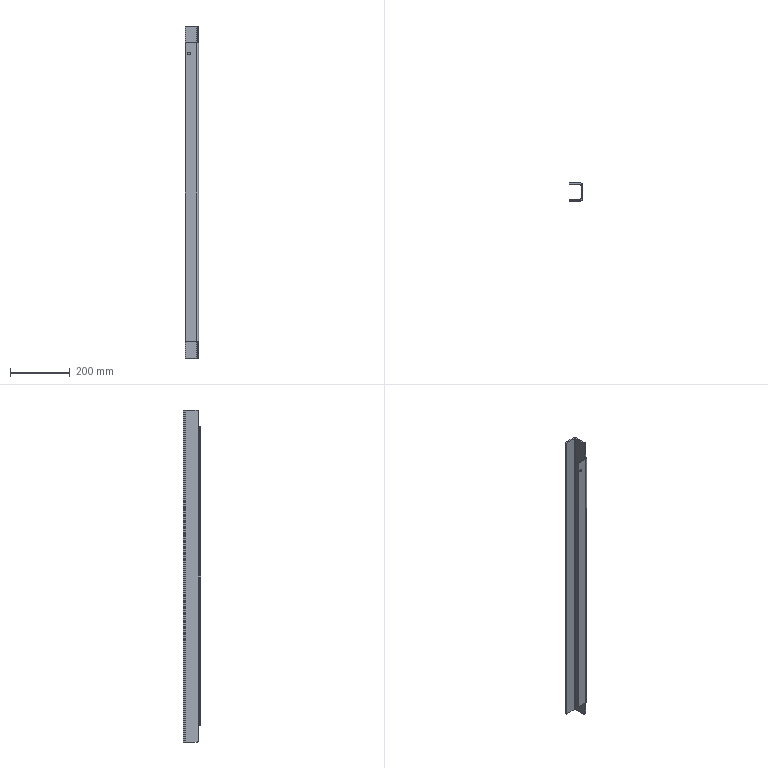Part | SolidWorks | features ICE 2, Extrusion 1, Fillet 1, HoleWzd 1 | 1 solid | 22 faces | box 45 x 60 x 1116 mm | volume 728504 mm3 | plane 14 | cylinder 8 | commonest cylinder face diameters 6 x2 8.5 x2 10 x2 16 x2
STEP:
#1=CARTESIAN_POINT('',(12.5,-60.,1028.25));
#2=VERTEX_POINT('',#1);
#3=CARTESIAN_POINT('',(12.5,-60.,1019.75));
#4=VERTEX_POINT('',#3);
#5=CARTESIAN_POINT('',(12.5,-60.,1024.));
#6=DIRECTION('',(0.,-1.,0.));
#7=DIRECTION('',(1.,0.,0.));
#8=AXIS2_PLACEMENT_3D('',#5,#6,#7);
#9=CIRCLE('',#8,4.25);
#10=EDGE_CURVE('',#2,#4,#9,.T.);
#11=ORIENTED_EDGE('',*,*,#10,.T.);
#12=CARTESIAN_POINT('',(12.5,-55.,1019.75));
#13=VERTEX_POINT('',#12);
#14=CARTESIAN_POINT('',(12.5,-55.,1019.75));
#15=DIRECTION('',(0.,1.,0.));
#16=VECTOR('',#15,1000.);
#17=LINE('',#14,#16);
#18=EDGE_CURVE('',#4,#13,#17,.T.);
#19=ORIENTED_EDGE('',*,*,#18,.T.);
#20=CARTESIAN_POINT('',(12.5,-55.,1028.25));
#21=VERTEX_POINT('',#20);
#22=CARTESIAN_POINT('',(12.5,-55.,1024.));
#23=DIRECTION('',(0.,1.,0.));
#24=DIRECTION('',(0.,0.,1.));
#25=AXIS2_PLACEMENT_3D('',#22,#23,#24);
#26=CIRCLE('',#25,4.25);
#27=EDGE_CURVE('',#13,#21,#26,.T.);
#28=ORIENTED_EDGE('',*,*,#27,.T.);
#29=CARTESIAN_POINT('',(12.5,-55.,1028.25));
#30=DIRECTION('',(0.,1.,0.));
#31=VECTOR('',#30,1000.);
#32=LINE('',#29,#31);
#33=EDGE_CURVE('',#2,#21,#32,.T.);
#34=ORIENTED_EDGE('',*,*,#33,.F.);
#35=EDGE_LOOP('',(#11,#19,#28,#34));
#36=FACE_OUTER_BOUND('',#35,.T.);
#37=CARTESIAN_POINT('',(12.5,-55.,1024.));
#38=DIRECTION('',(0.,1.,0.));
#39=DIRECTION('',(0.,0.,1.));
#40=AXIS2_PLACEMENT_3D('',#37,#38,#39);
#41=CYLINDRICAL_SURFACE('',#40,4.25);
#42=ADVANCED_FACE('',(#36),#41,.F.);
#43=CARTESIAN_POINT('',(12.5,-55.,1024.));
#44=DIRECTION('',(0.,1.,0.));
#45=DIRECTION('',(0.,0.,1.));
#46=AXIS2_PLACEMENT_3D('',#43,#44,#45);
#47=CIRCLE('',#46,4.25);
#48=EDGE_CURVE('',#21,#13,#47,.T.);
#49=ORIENTED_EDGE('',*,*,#48,.F.);
#50=ORIENTED_EDGE('',*,*,#27,.F.);
#51=EDGE_LOOP('',(#49,#50));
#52=FACE_BOUND('',#51,.T.);
#53=CARTESIAN_POINT('',(0.,-55.,1059.));
#54=VERTEX_POINT('',#53);
#55=CARTESIAN_POINT('',(0.,-55.,57.));
#56=VERTEX_POINT('',#55);
#57=CARTESIAN_POINT('',(0.,-55.,1116.));
#58=DIRECTION('',(0.,0.,-1.));
#59=VECTOR('',#58,1000.);
#60=LINE('',#57,#59);
#61=EDGE_CURVE('',#54,#56,#60,.T.);
#62=ORIENTED_EDGE('',*,*,#61,.F.);
#63=CARTESIAN_POINT('',(37.,-55.,1059.));
#64=VERTEX_POINT('',#63);
#65=CARTESIAN_POINT('',(37.,-55.,1059.));
#66=DIRECTION('',(1.,0.,0.));
#67=VECTOR('',#66,1000.);
#68=LINE('',#65,#67);
#69=EDGE_CURVE('',#54,#64,#68,.T.);
#70=ORIENTED_EDGE('',*,*,#69,.T.);
#71=CARTESIAN_POINT('',(37.,-55.,57.));
#72=VERTEX_POINT('',#71);
#73=CARTESIAN_POINT('',(37.,-55.,1116.));
#74=DIRECTION('',(0.,0.,-1.));
#75=VECTOR('',#74,1000.);
#76=LINE('',#73,#75);
#77=EDGE_CURVE('',#64,#72,#76,.T.);
#78=ORIENTED_EDGE('',*,*,#77,.T.);
#79=CARTESIAN_POINT('',(37.,-55.,57.));
#80=DIRECTION('',(-1.,0.,0.));
#81=VECTOR('',#80,1000.);
#82=LINE('',#79,#81);
#83=EDGE_CURVE('',#72,#56,#82,.T.);
#84=ORIENTED_EDGE('',*,*,#83,.T.);
#85=EDGE_LOOP('',(#62,#70,#78,#84));
#86=FACE_OUTER_BOUND('',#85,.T.);
#87=CARTESIAN_POINT('',(37.,-55.,1116.));
#88=DIRECTION('',(0.,-1.,0.));
#89=DIRECTION('',(0.,0.,-1.));
#90=AXIS2_PLACEMENT_3D('',#87,#88,#89);
#91=PLANE('',#90);
#92=ADVANCED_FACE('',(#52,#86),#91,.F.);
#93=CARTESIAN_POINT('',(0.,-60.,1059.));
#94=VERTEX_POINT('',#93);
#95=CARTESIAN_POINT('',(0.,-60.,57.));
#96=VERTEX_POINT('',#95);
#97=CARTESIAN_POINT('',(0.,-60.,1116.));
#98=DIRECTION('',(0.,0.,-1.));
#99=VECTOR('',#98,1000.);
#100=LINE('',#97,#99);
#101=EDGE_CURVE('',#94,#96,#100,.T.);
#102=ORIENTED_EDGE('',*,*,#101,.F.);
#103=CARTESIAN_POINT('',(0.,-52.,1059.));
#104=DIRECTION('',(0.,-1.,0.));
#105=VECTOR('',#104,1000.);
#106=LINE('',#103,#105);
#107=EDGE_CURVE('',#54,#94,#106,.T.);
#108=ORIENTED_EDGE('',*,*,#107,.F.);
#109=ORIENTED_EDGE('',*,*,#61,.T.);
#110=CARTESIAN_POINT('',(0.,-96.857,57.));
#111=DIRECTION('',(0.,1.,0.));
#112=VECTOR('',#111,1000.);
#113=LINE('',#110,#112);
#114=EDGE_CURVE('',#96,#56,#113,.T.);
#115=ORIENTED_EDGE('',*,*,#114,.F.);
#116=EDGE_LOOP('',(#102,#108,#109,#115));
#117=FACE_OUTER_BOUND('',#116,.T.);
#118=CARTESIAN_POINT('',(0.,-55.,1116.));
#119=DIRECTION('',(1.,0.,0.));
#120=DIRECTION('',(0.,0.,-1.));
#121=AXIS2_PLACEMENT_3D('',#118,#119,#120);
#122=PLANE('',#121);
#123=ADVANCED_FACE('',(#117),#122,.F.);
#124=ORIENTED_EDGE('',*,*,#10,.F.);
#125=CARTESIAN_POINT('',(12.5,-60.,1024.));
#126=DIRECTION('',(0.,-1.,0.));
#127=DIRECTION('',(1.,0.,0.));
#128=AXIS2_PLACEMENT_3D('',#125,#126,#127);
#129=CIRCLE('',#128,4.25);
#130=EDGE_CURVE('',#4,#2,#129,.T.);
#131=ORIENTED_EDGE('',*,*,#130,.F.);
#132=EDGE_LOOP('',(#124,#131));
#133=FACE_BOUND('',#132,.T.);
#134=CARTESIAN_POINT('',(37.,-60.,1059.));
#135=VERTEX_POINT('',#134);
#136=CARTESIAN_POINT('',(37.,-60.,1059.));
#137=DIRECTION('',(1.,0.,0.));
#138=VECTOR('',#137,1000.);
#139=LINE('',#136,#138);
#140=EDGE_CURVE('',#94,#135,#139,.T.);
#141=ORIENTED_EDGE('',*,*,#140,.F.);
#142=ORIENTED_EDGE('',*,*,#101,.T.);
#143=CARTESIAN_POINT('',(37.,-60.,57.));
#144=VERTEX_POINT('',#143);
#145=CARTESIAN_POINT('',(37.,-60.,57.));
#146=DIRECTION('',(-1.,0.,0.));
#147=VECTOR('',#146,1000.);
#148=LINE('',#145,#147);
#149=EDGE_CURVE('',#144,#96,#148,.T.);
#150=ORIENTED_EDGE('',*,*,#149,.F.);
#151=CARTESIAN_POINT('',(37.,-60.,1116.));
#152=DIRECTION('',(0.,0.,-1.));
#153=VECTOR('',#152,1000.);
#154=LINE('',#151,#153);
#155=EDGE_CURVE('',#135,#144,#154,.T.);
#156=ORIENTED_EDGE('',*,*,#155,.F.);
#157=EDGE_LOOP('',(#141,#142,#150,#156));
#158=FACE_OUTER_BOUND('',#157,.T.);
#159=CARTESIAN_POINT('',(37.,-60.,1116.));
#160=DIRECTION('',(0.,-1.,0.));
#161=DIRECTION('',(1.,0.,0.));
#162=AXIS2_PLACEMENT_3D('',#159,#160,#161);
#163=PLANE('',#162);
#164=ADVANCED_FACE('',(#133,#158),#163,.T.);
#165=CARTESIAN_POINT('',(45.,-52.,1059.));
#166=VERTEX_POINT('',#165);
#167=CARTESIAN_POINT('',(37.,-52.,1059.));
#168=DIRECTION('',(0.,0.,1.));
#169=DIRECTION('',(-1.,0.,0.));
#170=AXIS2_PLACEMENT_3D('',#167,#168,#169);
#171=CIRCLE('',#170,8.);
#172=EDGE_CURVE('',#135,#166,#171,.T.);
#173=ORIENTED_EDGE('',*,*,#172,.F.);
#174=ORIENTED_EDGE('',*,*,#155,.T.);
#175=CARTESIAN_POINT('',(45.,-52.,57.));
#176=VERTEX_POINT('',#175);
#177=CARTESIAN_POINT('',(37.,-52.,57.));
#178=DIRECTION('',(0.,0.,-1.));
#179=DIRECTION('',(1.,0.,0.));
#180=AXIS2_PLACEMENT_3D('',#177,#178,#179);
#181=CIRCLE('',#180,8.);
#182=EDGE_CURVE('',#176,#144,#181,.T.);
#183=ORIENTED_EDGE('',*,*,#182,.F.);
#184=CARTESIAN_POINT('',(45.,-52.,1116.));
#185=DIRECTION('',(0.,0.,-1.));
#186=VECTOR('',#185,1000.);
#187=LINE('',#184,#186);
#188=EDGE_CURVE('',#166,#176,#187,.T.);
#189=ORIENTED_EDGE('',*,*,#188,.F.);
#190=EDGE_LOOP('',(#173,#174,#183,#189));
#191=FACE_OUTER_BOUND('',#190,.T.);
#192=CARTESIAN_POINT('',(37.,-52.,1116.));
#193=DIRECTION('',(0.,0.,-1.));
#194=DIRECTION('',(-1.,0.,0.));
#195=AXIS2_PLACEMENT_3D('',#192,#193,#194);
#196=CYLINDRICAL_SURFACE('',#195,8.);
#197=ADVANCED_FACE('',(#191),#196,.T.);
#198=CARTESIAN_POINT('',(45.,-8.,1116.));
#199=VERTEX_POINT('',#198);
#200=CARTESIAN_POINT('',(45.,-47.,1116.));
#201=VERTEX_POINT('',#200);
#202=CARTESIAN_POINT('',(45.,-8.,1116.));
#203=DIRECTION('',(0.,-1.,0.));
#204=VECTOR('',#203,1000.);
#205=LINE('',#202,#204);
#206=EDGE_CURVE('',#199,#201,#205,.T.);
#207=ORIENTED_EDGE('',*,*,#206,.T.);
#208=CARTESIAN_POINT('',(45.,-52.,1111.));
#209=VERTEX_POINT('',#208);
#210=CARTESIAN_POINT('',(45.,-47.,1111.));
#211=DIRECTION('',(1.,0.,0.));
#212=DIRECTION('',(0.,1.,0.));
#213=AXIS2_PLACEMENT_3D('',#210,#211,#212);
#214=CIRCLE('',#213,5.);
#215=EDGE_CURVE('',#201,#209,#214,.T.);
#216=ORIENTED_EDGE('',*,*,#215,.T.);
#217=CARTESIAN_POINT('',(45.,-52.,1116.));
#218=DIRECTION('',(0.,0.,-1.));
#219=VECTOR('',#218,1000.);
#220=LINE('',#217,#219);
#221=EDGE_CURVE('',#209,#166,#220,.T.);
#222=ORIENTED_EDGE('',*,*,#221,.T.);
#223=ORIENTED_EDGE('',*,*,#188,.T.);
#224=CARTESIAN_POINT('',(45.,-52.,5.));
#225=VERTEX_POINT('',#224);
#226=CARTESIAN_POINT('',(45.,-52.,1116.));
#227=DIRECTION('',(0.,0.,1.));
#228=VECTOR('',#227,1000.);
#229=LINE('',#226,#228);
#230=EDGE_CURVE('',#225,#176,#229,.T.);
#231=ORIENTED_EDGE('',*,*,#230,.F.);
#232=CARTESIAN_POINT('',(45.,-47.,0.));
#233=VERTEX_POINT('',#232);
#234=CARTESIAN_POINT('',(45.,-47.,5.));
#235=DIRECTION('',(1.,0.,0.));
#236=DIRECTION('',(0.,1.,0.));
#237=AXIS2_PLACEMENT_3D('',#234,#235,#236);
#238=CIRCLE('',#237,5.);
#239=EDGE_CURVE('',#225,#233,#238,.T.);
#240=ORIENTED_EDGE('',*,*,#239,.T.);
#241=CARTESIAN_POINT('',(45.,-8.,0.));
#242=VERTEX_POINT('',#241);
#243=CARTESIAN_POINT('',(45.,-8.,0.));
#244=DIRECTION('',(0.,-1.,0.));
#245=VECTOR('',#244,1000.);
#246=LINE('',#243,#245);
#247=EDGE_CURVE('',#242,#233,#246,.T.);
#248=ORIENTED_EDGE('',*,*,#247,.F.);
#249=CARTESIAN_POINT('',(45.,-8.,1116.));
#250=DIRECTION('',(0.,0.,-1.));
#251=VECTOR('',#250,1000.);
#252=LINE('',#249,#251);
#253=EDGE_CURVE('',#199,#242,#252,.T.);
#254=ORIENTED_EDGE('',*,*,#253,.F.);
#255=EDGE_LOOP('',(#207,#216,#222,#223,#231,#240,#248,#254));
#256=FACE_OUTER_BOUND('',#255,.T.);
#257=CARTESIAN_POINT('',(45.,-8.,1116.));
#258=DIRECTION('',(1.,0.,0.));
#259=DIRECTION('',(0.,1.,0.));
#260=AXIS2_PLACEMENT_3D('',#257,#258,#259);
#261=PLANE('',#260);
#262=ADVANCED_FACE('',(#256),#261,.T.);
#263=CARTESIAN_POINT('',(37.,0.,0.));
#264=VERTEX_POINT('',#263);
#265=CARTESIAN_POINT('',(37.,-8.,0.));
#266=DIRECTION('',(0.,0.,-1.));
#267=DIRECTION('',(-1.,0.,0.));
#268=AXIS2_PLACEMENT_3D('',#265,#266,#267);
#269=CIRCLE('',#268,8.);
#270=EDGE_CURVE('',#264,#242,#269,.T.);
#271=ORIENTED_EDGE('',*,*,#270,.F.);
#272=CARTESIAN_POINT('',(37.,0.,1116.));
#273=VERTEX_POINT('',#272);
#274=CARTESIAN_POINT('',(37.,0.,1116.));
#275=DIRECTION('',(0.,0.,-1.));
#276=VECTOR('',#275,1000.);
#277=LINE('',#274,#276);
#278=EDGE_CURVE('',#273,#264,#277,.T.);
#279=ORIENTED_EDGE('',*,*,#278,.F.);
#280=CARTESIAN_POINT('',(37.,-8.,1116.));
#281=DIRECTION('',(0.,0.,-1.));
#282=DIRECTION('',(-1.,0.,0.));
#283=AXIS2_PLACEMENT_3D('',#280,#281,#282);
#284=CIRCLE('',#283,8.);
#285=EDGE_CURVE('',#273,#199,#284,.T.);
#286=ORIENTED_EDGE('',*,*,#285,.T.);
#287=ORIENTED_EDGE('',*,*,#253,.T.);
#288=EDGE_LOOP('',(#271,#279,#286,#287));
#289=FACE_OUTER_BOUND('',#288,.T.);
#290=CARTESIAN_POINT('',(37.,-8.,1116.));
#291=DIRECTION('',(0.,0.,-1.));
#292=DIRECTION('',(-1.,0.,0.));
#293=AXIS2_PLACEMENT_3D('',#290,#291,#292);
#294=CYLINDRICAL_SURFACE('',#293,8.);
#295=ADVANCED_FACE('',(#289),#294,.T.);
#296=CARTESIAN_POINT('',(0.,0.,0.));
#297=VERTEX_POINT('',#296);
#298=CARTESIAN_POINT('',(0.,0.,0.));
#299=DIRECTION('',(1.,0.,0.));
#300=VECTOR('',#299,1000.);
#301=LINE('',#298,#300);
#302=EDGE_CURVE('',#297,#264,#301,.T.);
#303=ORIENTED_EDGE('',*,*,#302,.F.);
#304=CARTESIAN_POINT('',(0.,0.,1116.));
#305=VERTEX_POINT('',#304);
#306=CARTESIAN_POINT('',(0.,0.,1116.));
#307=DIRECTION('',(0.,0.,-1.));
#308=VECTOR('',#307,1000.);
#309=LINE('',#306,#308);
#310=EDGE_CURVE('',#305,#297,#309,.T.);
#311=ORIENTED_EDGE('',*,*,#310,.F.);
#312=CARTESIAN_POINT('',(0.,0.,1116.));
#313=DIRECTION('',(1.,0.,0.));
#314=VECTOR('',#313,1000.);
#315=LINE('',#312,#314);
#316=EDGE_CURVE('',#305,#273,#315,.T.);
#317=ORIENTED_EDGE('',*,*,#316,.T.);
#318=ORIENTED_EDGE('',*,*,#278,.T.);
#319=EDGE_LOOP('',(#303,#311,#317,#318));
#320=FACE_OUTER_BOUND('',#319,.T.);
#321=CARTESIAN_POINT('',(0.,0.,1116.));
#322=DIRECTION('',(0.,1.,0.));
#323=DIRECTION('',(0.,0.,1.));
#324=AXIS2_PLACEMENT_3D('',#321,#322,#323);
#325=PLANE('',#324);
#326=ADVANCED_FACE('',(#320),#325,.T.);
#327=CARTESIAN_POINT('',(0.,-5.,0.));
#328=VERTEX_POINT('',#327);
#329=CARTESIAN_POINT('',(0.,0.,0.));
#330=DIRECTION('',(0.,-1.,0.));
#331=VECTOR('',#330,1000.);
#332=LINE('',#329,#331);
#333=EDGE_CURVE('',#297,#328,#332,.T.);
#334=ORIENTED_EDGE('',*,*,#333,.T.);
#335=CARTESIAN_POINT('',(0.,-5.,1116.));
#336=VERTEX_POINT('',#335);
#337=CARTESIAN_POINT('',(0.,-5.,1116.));
#338=DIRECTION('',(0.,0.,-1.));
#339=VECTOR('',#338,1000.);
#340=LINE('',#337,#339);
#341=EDGE_CURVE('',#336,#328,#340,.T.);
#342=ORIENTED_EDGE('',*,*,#341,.F.);
#343=CARTESIAN_POINT('',(0.,0.,1116.));
#344=DIRECTION('',(0.,-1.,0.));
#345=VECTOR('',#344,1000.);
#346=LINE('',#343,#345);
#347=EDGE_CURVE('',#305,#336,#346,.T.);
#348=ORIENTED_EDGE('',*,*,#347,.F.);
#349=ORIENTED_EDGE('',*,*,#310,.T.);
#350=EDGE_LOOP('',(#334,#342,#348,#349));
#351=FACE_OUTER_BOUND('',#350,.T.);
#352=CARTESIAN_POINT('',(0.,0.,1116.));
#353=DIRECTION('',(1.,0.,0.));
#354=DIRECTION('',(0.,0.,-1.));
#355=AXIS2_PLACEMENT_3D('',#352,#353,#354);
#356=PLANE('',#355);
#357=ADVANCED_FACE('',(#351),#356,.F.);
#358=CARTESIAN_POINT('',(37.,-5.,0.));
#359=VERTEX_POINT('',#358);
#360=CARTESIAN_POINT('',(0.,-5.,0.));
#361=DIRECTION('',(1.,0.,0.));
#362=VECTOR('',#361,1000.);
#363=LINE('',#360,#362);
#364=EDGE_CURVE('',#328,#359,#363,.T.);
#365=ORIENTED_EDGE('',*,*,#364,.T.);
#366=CARTESIAN_POINT('',(37.,-5.,1116.));
#367=VERTEX_POINT('',#366);
#368=CARTESIAN_POINT('',(37.,-5.,1116.));
#369=DIRECTION('',(0.,0.,-1.));
#370=VECTOR('',#369,1000.);
#371=LINE('',#368,#370);
#372=EDGE_CURVE('',#367,#359,#371,.T.);
#373=ORIENTED_EDGE('',*,*,#372,.F.);
#374=CARTESIAN_POINT('',(0.,-5.,1116.));
#375=DIRECTION('',(1.,0.,0.));
#376=VECTOR('',#375,1000.);
#377=LINE('',#374,#376);
#378=EDGE_CURVE('',#336,#367,#377,.T.);
#379=ORIENTED_EDGE('',*,*,#378,.F.);
#380=ORIENTED_EDGE('',*,*,#341,.T.);
#381=EDGE_LOOP('',(#365,#373,#379,#380));
#382=FACE_OUTER_BOUND('',#381,.T.);
#383=CARTESIAN_POINT('',(0.,-5.,1116.));
#384=DIRECTION('',(0.,1.,0.));
#385=DIRECTION('',(0.,0.,1.));
#386=AXIS2_PLACEMENT_3D('',#383,#384,#385);
#387=PLANE('',#386);
#388=ADVANCED_FACE('',(#382),#387,.F.);
#389=CARTESIAN_POINT('',(40.,-8.,0.));
#390=VERTEX_POINT('',#389);
#391=CARTESIAN_POINT('',(37.,-8.,0.));
#392=DIRECTION('',(0.,0.,-1.));
#393=DIRECTION('',(-1.,0.,0.));
#394=AXIS2_PLACEMENT_3D('',#391,#392,#393);
#395=CIRCLE('',#394,3.);
#396=EDGE_CURVE('',#359,#390,#395,.T.);
#397=ORIENTED_EDGE('',*,*,#396,.T.);
#398=CARTESIAN_POINT('',(40.,-8.,1116.));
#399=VERTEX_POINT('',#398);
#400=CARTESIAN_POINT('',(40.,-8.,1116.));
#401=DIRECTION('',(0.,0.,-1.));
#402=VECTOR('',#401,1000.);
#403=LINE('',#400,#402);
#404=EDGE_CURVE('',#399,#390,#403,.T.);
#405=ORIENTED_EDGE('',*,*,#404,.F.);
#406=CARTESIAN_POINT('',(37.,-8.,1116.));
#407=DIRECTION('',(0.,0.,-1.));
#408=DIRECTION('',(-1.,0.,0.));
#409=AXIS2_PLACEMENT_3D('',#406,#407,#408);
#410=CIRCLE('',#409,3.);
#411=EDGE_CURVE('',#367,#399,#410,.T.);
#412=ORIENTED_EDGE('',*,*,#411,.F.);
#413=ORIENTED_EDGE('',*,*,#372,.T.);
#414=EDGE_LOOP('',(#397,#405,#412,#413));
#415=FACE_OUTER_BOUND('',#414,.T.);
#416=CARTESIAN_POINT('',(37.,-8.,1116.));
#417=DIRECTION('',(0.,0.,-1.));
#418=DIRECTION('',(-1.,0.,0.));
#419=AXIS2_PLACEMENT_3D('',#416,#417,#418);
#420=CYLINDRICAL_SURFACE('',#419,3.);
#421=ADVANCED_FACE('',(#415),#420,.F.);
#422=CARTESIAN_POINT('',(40.,-52.,1111.));
#423=VERTEX_POINT('',#422);
#424=CARTESIAN_POINT('',(40.,-52.,1059.));
#425=VERTEX_POINT('',#424);
#426=CARTESIAN_POINT('',(40.,-52.,1116.));
#427=DIRECTION('',(0.,0.,-1.));
#428=VECTOR('',#427,1000.);
#429=LINE('',#426,#428);
#430=EDGE_CURVE('',#423,#425,#429,.T.);
#431=ORIENTED_EDGE('',*,*,#430,.F.);
#432=CARTESIAN_POINT('',(40.,-47.,1116.));
#433=VERTEX_POINT('',#432);
#434=CARTESIAN_POINT('',(40.,-47.,1111.));
#435=DIRECTION('',(-1.,0.,0.));
#436=DIRECTION('',(0.,0.,-1.));
#437=AXIS2_PLACEMENT_3D('',#434,#435,#436);
#438=CIRCLE('',#437,5.);
#439=EDGE_CURVE('',#423,#433,#438,.T.);
#440=ORIENTED_EDGE('',*,*,#439,.T.);
#441=CARTESIAN_POINT('',(40.,-8.,1116.));
#442=DIRECTION('',(0.,-1.,0.));
#443=VECTOR('',#442,1000.);
#444=LINE('',#441,#443);
#445=EDGE_CURVE('',#399,#433,#444,.T.);
#446=ORIENTED_EDGE('',*,*,#445,.F.);
#447=ORIENTED_EDGE('',*,*,#404,.T.);
#448=CARTESIAN_POINT('',(40.,-47.,0.));
#449=VERTEX_POINT('',#448);
#450=CARTESIAN_POINT('',(40.,-8.,0.));
#451=DIRECTION('',(0.,-1.,0.));
#452=VECTOR('',#451,1000.);
#453=LINE('',#450,#452);
#454=EDGE_CURVE('',#390,#449,#453,.T.);
#455=ORIENTED_EDGE('',*,*,#454,.T.);
#456=CARTESIAN_POINT('',(40.,-52.,5.));
#457=VERTEX_POINT('',#456);
#458=CARTESIAN_POINT('',(40.,-47.,5.));
#459=DIRECTION('',(-1.,0.,0.));
#460=DIRECTION('',(0.,0.,-1.));
#461=AXIS2_PLACEMENT_3D('',#458,#459,#460);
#462=CIRCLE('',#461,5.);
#463=EDGE_CURVE('',#449,#457,#462,.T.);
#464=ORIENTED_EDGE('',*,*,#463,.T.);
#465=CARTESIAN_POINT('',(40.,-52.,57.));
#466=VERTEX_POINT('',#465);
#467=CARTESIAN_POINT('',(40.,-52.,1116.));
#468=DIRECTION('',(0.,0.,1.));
#469=VECTOR('',#468,1000.);
#470=LINE('',#467,#469);
#471=EDGE_CURVE('',#457,#466,#470,.T.);
#472=ORIENTED_EDGE('',*,*,#471,.T.);
#473=CARTESIAN_POINT('',(40.,-52.,1116.));
#474=DIRECTION('',(0.,0.,-1.));
#475=VECTOR('',#474,1000.);
#476=LINE('',#473,#475);
#477=EDGE_CURVE('',#425,#466,#476,.T.);
#478=ORIENTED_EDGE('',*,*,#477,.F.);
#479=EDGE_LOOP('',(#431,#440,#446,#447,#455,#464,#472,#478));
#480=FACE_OUTER_BOUND('',#479,.T.);
#481=CARTESIAN_POINT('',(40.,-8.,1116.));
#482=DIRECTION('',(1.,0.,0.));
#483=DIRECTION('',(0.,0.,-1.));
#484=AXIS2_PLACEMENT_3D('',#481,#482,#483);
#485=PLANE('',#484);
#486=ADVANCED_FACE('',(#480),#485,.F.);
#487=ORIENTED_EDGE('',*,*,#77,.F.);
#488=CARTESIAN_POINT('',(37.,-52.,1059.));
#489=DIRECTION('',(0.,0.,1.));
#490=DIRECTION('',(-1.,0.,0.));
#491=AXIS2_PLACEMENT_3D('',#488,#489,#490);
#492=CIRCLE('',#491,3.);
#493=EDGE_CURVE('',#64,#425,#492,.T.);
#494=ORIENTED_EDGE('',*,*,#493,.T.);
#495=ORIENTED_EDGE('',*,*,#477,.T.);
#496=CARTESIAN_POINT('',(37.,-52.,57.));
#497=DIRECTION('',(0.,0.,-1.));
#498=DIRECTION('',(1.,0.,0.));
#499=AXIS2_PLACEMENT_3D('',#496,#497,#498);
#500=CIRCLE('',#499,3.);
#501=EDGE_CURVE('',#466,#72,#500,.T.);
#502=ORIENTED_EDGE('',*,*,#501,.T.);
#503=EDGE_LOOP('',(#487,#494,#495,#502));
#504=FACE_OUTER_BOUND('',#503,.T.);
#505=CARTESIAN_POINT('',(37.,-52.,1116.));
#506=DIRECTION('',(0.,0.,-1.));
#507=DIRECTION('',(-1.,0.,0.));
#508=AXIS2_PLACEMENT_3D('',#505,#506,#507);
#509=CYLINDRICAL_SURFACE('',#508,3.);
#510=ADVANCED_FACE('',(#504),#509,.F.);
#511=ORIENTED_EDGE('',*,*,#445,.T.);
#512=CARTESIAN_POINT('',(37.,-47.,1116.));
#513=DIRECTION('',(1.,0.,0.));
#514=VECTOR('',#513,1000.);
#515=LINE('',#512,#514);
#516=EDGE_CURVE('',#433,#201,#515,.T.);
#517=ORIENTED_EDGE('',*,*,#516,.T.);
#518=ORIENTED_EDGE('',*,*,#206,.F.);
#519=ORIENTED_EDGE('',*,*,#285,.F.);
#520=ORIENTED_EDGE('',*,*,#316,.F.);
#521=ORIENTED_EDGE('',*,*,#347,.T.);
#522=ORIENTED_EDGE('',*,*,#378,.T.);
#523=ORIENTED_EDGE('',*,*,#411,.T.);
#524=EDGE_LOOP('',(#511,#517,#518,#519,#520,#521,#522,#523));
#525=FACE_OUTER_BOUND('',#524,.T.);
#526=CARTESIAN_POINT('',(37.,-52.,1116.));
#527=DIRECTION('',(0.,0.,-1.));
#528=DIRECTION('',(-1.,0.,0.));
#529=AXIS2_PLACEMENT_3D('',#526,#527,#528);
#530=PLANE('',#529);
#531=ADVANCED_FACE('',(#525),#530,.F.);
#532=ORIENTED_EDGE('',*,*,#247,.T.);
#533=CARTESIAN_POINT('',(40.,-47.,0.));
#534=DIRECTION('',(-1.,0.,0.));
#535=VECTOR('',#534,1000.);
#536=LINE('',#533,#535);
#537=EDGE_CURVE('',#233,#449,#536,.T.);
#538=ORIENTED_EDGE('',*,*,#537,.T.);
#539=ORIENTED_EDGE('',*,*,#454,.F.);
#540=ORIENTED_EDGE('',*,*,#396,.F.);
#541=ORIENTED_EDGE('',*,*,#364,.F.);
#542=ORIENTED_EDGE('',*,*,#333,.F.);
#543=ORIENTED_EDGE('',*,*,#302,.T.);
#544=ORIENTED_EDGE('',*,*,#270,.T.);
#545=EDGE_LOOP('',(#532,#538,#539,#540,#541,#542,#543,#544));
#546=FACE_OUTER_BOUND('',#545,.T.);
#547=CARTESIAN_POINT('',(37.,-52.,0.));
#548=DIRECTION('',(0.,0.,-1.));
#549=DIRECTION('',(-1.,0.,0.));
#550=AXIS2_PLACEMENT_3D('',#547,#548,#549);
#551=PLANE('',#550);
#552=ADVANCED_FACE('',(#546),#551,.T.);
#553=ORIENTED_EDGE('',*,*,#149,.T.);
#554=ORIENTED_EDGE('',*,*,#114,.T.);
#555=ORIENTED_EDGE('',*,*,#83,.F.);
#556=ORIENTED_EDGE('',*,*,#501,.F.);
#557=CARTESIAN_POINT('',(1116.,-52.,57.));
#558=DIRECTION('',(-1.,0.,0.));
#559=VECTOR('',#558,1000.);
#560=LINE('',#557,#559);
#561=EDGE_CURVE('',#176,#466,#560,.T.);
#562=ORIENTED_EDGE('',*,*,#561,.F.);
#563=ORIENTED_EDGE('',*,*,#182,.T.);
#564=EDGE_LOOP('',(#553,#554,#555,#556,#562,#563));
#565=FACE_OUTER_BOUND('',#564,.T.);
#566=CARTESIAN_POINT('',(1116.,-96.857,57.));
#567=DIRECTION('',(0.,0.,1.));
#568=DIRECTION('',(1.,0.,0.));
#569=AXIS2_PLACEMENT_3D('',#566,#567,#568);
#570=PLANE('',#569);
#571=ADVANCED_FACE('',(#565),#570,.F.);
#572=ORIENTED_EDGE('',*,*,#471,.F.);
#573=CARTESIAN_POINT('',(45.,-52.,5.));
#574=DIRECTION('',(1.,0.,0.));
#575=VECTOR('',#574,1000.);
#576=LINE('',#573,#575);
#577=EDGE_CURVE('',#457,#225,#576,.T.);
#578=ORIENTED_EDGE('',*,*,#577,.T.);
#579=ORIENTED_EDGE('',*,*,#230,.T.);
#580=ORIENTED_EDGE('',*,*,#561,.T.);
#581=EDGE_LOOP('',(#572,#578,#579,#580));
#582=FACE_OUTER_BOUND('',#581,.T.);
#583=CARTESIAN_POINT('',(1116.,-52.,57.));
#584=DIRECTION('',(0.,1.,0.));
#585=DIRECTION('',(0.,0.,1.));
#586=AXIS2_PLACEMENT_3D('',#583,#584,#585);
#587=PLANE('',#586);
#588=ADVANCED_FACE('',(#582),#587,.F.);
#589=ORIENTED_EDGE('',*,*,#140,.T.);
#590=ORIENTED_EDGE('',*,*,#172,.T.);
#591=CARTESIAN_POINT('',(1116.,-52.,1059.));
#592=DIRECTION('',(-1.,0.,0.));
#593=VECTOR('',#592,1000.);
#594=LINE('',#591,#593);
#595=EDGE_CURVE('',#166,#425,#594,.T.);
#596=ORIENTED_EDGE('',*,*,#595,.T.);
#597=ORIENTED_EDGE('',*,*,#493,.F.);
#598=ORIENTED_EDGE('',*,*,#69,.F.);
#599=ORIENTED_EDGE('',*,*,#107,.T.);
#600=EDGE_LOOP('',(#589,#590,#596,#597,#598,#599));
#601=FACE_OUTER_BOUND('',#600,.T.);
#602=CARTESIAN_POINT('',(1116.,-52.,1059.));
#603=DIRECTION('',(0.,0.,-1.));
#604=DIRECTION('',(-1.,0.,0.));
#605=AXIS2_PLACEMENT_3D('',#602,#603,#604);
#606=PLANE('',#605);
#607=ADVANCED_FACE('',(#601),#606,.F.);
#608=ORIENTED_EDGE('',*,*,#221,.F.);
#609=CARTESIAN_POINT('',(1116.,-52.,1111.));
#610=DIRECTION('',(-1.,0.,0.));
#611=VECTOR('',#610,1000.);
#612=LINE('',#609,#611);
#613=EDGE_CURVE('',#209,#423,#612,.T.);
#614=ORIENTED_EDGE('',*,*,#613,.T.);
#615=ORIENTED_EDGE('',*,*,#430,.T.);
#616=ORIENTED_EDGE('',*,*,#595,.F.);
#617=EDGE_LOOP('',(#608,#614,#615,#616));
#618=FACE_OUTER_BOUND('',#617,.T.);
#619=CARTESIAN_POINT('',(1116.,-52.,1059.));
#620=DIRECTION('',(0.,1.,0.));
#621=DIRECTION('',(0.,0.,1.));
#622=AXIS2_PLACEMENT_3D('',#619,#620,#621);
#623=PLANE('',#622);
#624=ADVANCED_FACE('',(#618),#623,.F.);
#625=ORIENTED_EDGE('',*,*,#439,.F.);
#626=ORIENTED_EDGE('',*,*,#613,.F.);
#627=ORIENTED_EDGE('',*,*,#215,.F.);
#628=ORIENTED_EDGE('',*,*,#516,.F.);
#629=EDGE_LOOP('',(#625,#626,#627,#628));
#630=FACE_OUTER_BOUND('',#629,.T.);
#631=CARTESIAN_POINT('',(37.,-47.,1111.));
#632=DIRECTION('',(1.,0.,0.));
#633=DIRECTION('',(0.,0.,-1.));
#634=AXIS2_PLACEMENT_3D('',#631,#632,#633);
#635=CYLINDRICAL_SURFACE('',#634,5.);
#636=ADVANCED_FACE('',(#630),#635,.T.);
#637=ORIENTED_EDGE('',*,*,#463,.F.);
#638=ORIENTED_EDGE('',*,*,#537,.F.);
#639=ORIENTED_EDGE('',*,*,#239,.F.);
#640=ORIENTED_EDGE('',*,*,#577,.F.);
#641=EDGE_LOOP('',(#637,#638,#639,#640));
#642=FACE_OUTER_BOUND('',#641,.T.);
#643=CARTESIAN_POINT('',(1116.,-47.,5.));
#644=DIRECTION('',(-1.,0.,0.));
#645=DIRECTION('',(0.,0.,1.));
#646=AXIS2_PLACEMENT_3D('',#643,#644,#645);
#647=CYLINDRICAL_SURFACE('',#646,5.);
#648=ADVANCED_FACE('',(#642),#647,.T.);
#649=ORIENTED_EDGE('',*,*,#18,.F.);
#650=ORIENTED_EDGE('',*,*,#130,.T.);
#651=ORIENTED_EDGE('',*,*,#33,.T.);
#652=ORIENTED_EDGE('',*,*,#48,.T.);
#653=EDGE_LOOP('',(#649,#650,#651,#652));
#654=FACE_OUTER_BOUND('',#653,.T.);
#655=CARTESIAN_POINT('',(12.5,-55.,1024.));
#656=DIRECTION('',(0.,1.,0.));
#657=DIRECTION('',(0.,0.,1.));
#658=AXIS2_PLACEMENT_3D('',#655,#656,#657);
#659=CYLINDRICAL_SURFACE('',#658,4.25);
#660=ADVANCED_FACE('',(#654),#659,.F.);
#661=CLOSED_SHELL('',(#42,#92,#123,#164,#197,#262,#295,#326,#357,#388,#421,#486,#510,#531,#552,#571,#588,#607,#624,#636,#648,#660));
#662=MANIFOLD_SOLID_BREP('',#661);
#663=CARTESIAN_POINT('',(0.,0.,0.));
#664=DIRECTION('',(0.,0.,1.));
#665=DIRECTION('',(1.,0.,0.));
#666=AXIS2_PLACEMENT_3D('',#663,#664,#665);
#667=(LENGTH_UNIT()NAMED_UNIT(*)SI_UNIT(.MILLI.,.METRE.));
#668=UNCERTAINTY_MEASURE_WITH_UNIT(LENGTH_MEASURE(0.00001),#667,'','');
#669=(NAMED_UNIT(*)PLANE_ANGLE_UNIT()SI_UNIT($,.RADIAN.));
#670=(NAMED_UNIT(*)SI_UNIT($,.STERADIAN.)SOLID_ANGLE_UNIT());
#671=(GEOMETRIC_REPRESENTATION_CONTEXT(3)GLOBAL_UNCERTAINTY_ASSIGNED_CONTEXT((#668))GLOBAL_UNIT_ASSIGNED_CONTEXT((#667,#669,#670))REPRESENTATION_CONTEXT('',''));
#672=ADVANCED_BREP_SHAPE_REPRESENTATION('',(#662,#666),#671);